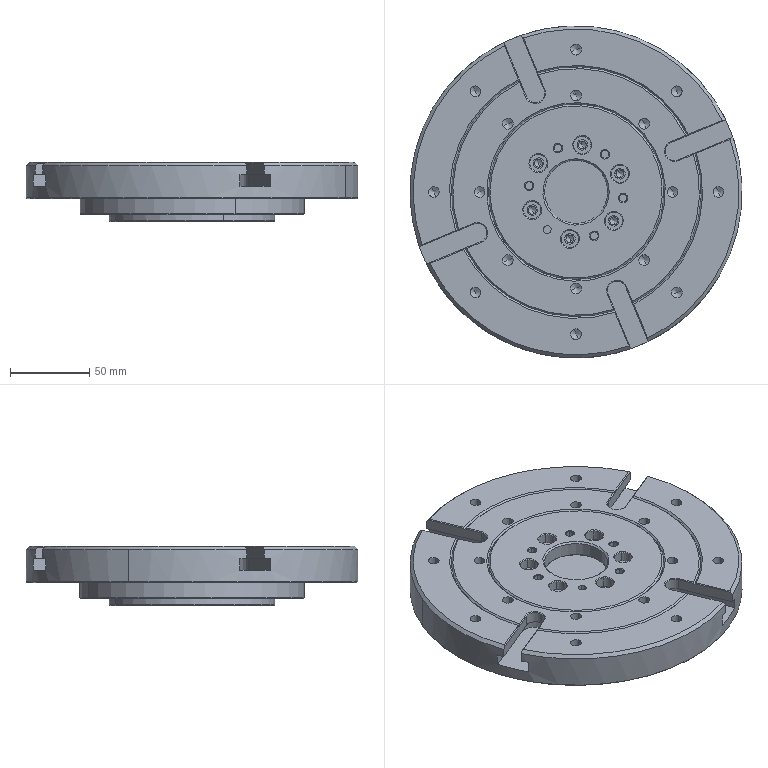NC program | Mastercam | posted with a generic post
Lines 1 to 724 of 4738:
%
:0001()
(MATERIAL - ALUMINUM MM - 2024)
(T1|8 FEMR |H1|XY STOCK TO LEAVE - .1|Z STOCK TO LEAVE - 0.)
(T2|2.5 DR |H2)
(T5|4 FEMR |H5|D5|WEAR COMP|TOOL DIA. - 4.|XY STOCK TO LEAVE - .1|Z STOCK TO LEAVE - .1)
(T6|2 FEMR |H6|D6|WEAR COMP|TOOL DIA. - 2.|XY STOCK TO LEAVE - .1|Z STOCK TO LEAVE - .1)
(T9|8 FEMF |H9|D9|WEAR COMP|TOOL DIA. - 8.)
(T10|12 R0.8 |H10)
(T7|2 FEMF |H7|D7|WEAR COMP|TOOL DIA. - 2.|XY STOCK TO LEAVE - 0.|Z STOCK TO LEAVE - .05)
(T8|6 XXXX |H8|D8|WEAR COMP|TOOL DIA. - 6.)
(T12|5 CHM |H12)
(T13|2.1 DR |H13)
(T11|3 FEM |H11)
(T14|1.95 THML |H14|D14|WEAR COMP|TOOL DIA. - 1.95)
(T15|2.5 BM |H15)
N100 G21
N102 G0 G17 G40 G80 G90 G94 G98
N104 G0 G28 G91 Z0.
N106 G0 G28 X0. Y0.
(8 FEMR |TOOL - 1|DIA. OFF. - 1|LEN. - 1|TOOL DIA. - 8.)
N108 T1 M6
N110 G0 G54 G90 X15.985 Y3.58 C0. B0. S3500 M3
N112 G43 H1 Z50.
N114 Z13.45
N116 G1 Z4.7 F2000.
N118 X15.936 Y3.498
N120 X15.057 Y2.03 Z4.53
N122 G3 X14.809 Y1.274 Z4.45 I1.544 J-.925
N124 X14.755 Y.115 I12.301 J-1.159
N126 X14.754 Y.062 I12.355
N128 G1 Y.045
N130 G2 X14.688 Y-.692 I-4.1
N132 G3 X14.685 Y-.704 I.786 J-.144
N134 G2 X14.583 Y-1.29 I-79.757 J13.658
N136 G1 X14.534 Y-1.568
N138 G2 X14.201 Y-3.41 I-70.503 J11.78
N140 X11.76 Y-8.452 I-16.311 J4.785
N142 X.007 Y-14.474 I-11.753 J8.459
N144 X-14.474 Y.007 J14.481
N146 G1 X-14.473 Y.164
N148 G2 X-13.125 Y6.103 I14.466 J-.163
N150 G3 X-13.06 Y6.318 I-.726 J.338
N152 G2 X-12.476 Y7.877 I4.051 J-.63
N154 G3 X-12.185 Y8.362 I-10.447 J6.598
N156 X-11.954 Y9.123 Z4.53 I-1.564 J.89
N158 G1 X-11.832 Y10.83 Z4.7
N160 X-11.825 Y10.926
N162 G3 X-11.824 Y10.967 I-.578 J.041 F9500.
N164 X-12.403 Y11.546 I-.579
N166 G1 X-12.572 Y11.521
N168 X-12.726 Y11.448
N170 X-12.853 Y11.333
N172 X-12.94 Y11.185
N174 X-14.656 Y6.988
N176 G3 X-15.882 Y.742 I15.291 J-6.246
N178 X.635 Y-15.775 I16.517
N180 X13.322 Y-9.835 J16.517
N182 G1 X18.397 Y-3.748
N184 G3 X18.604 Y-3.177 I-.685 J.571
N186 X18.049 Y-2.351 I-.892
N188 G1 X16.228 Y-1.606
N190 G3 X15.89 Y-1.54 I-.338 J-.826
N192 X15.794 Y-1.545 J-.892
N194 X15.196 Y-1.872 Z4.63 I.096 J-.887 F2000.
N196 G1 X14.561 Y-2.659 Z4.53
N198 G3 X14.21 Y-3.373 Z4.45 I1.401 J-1.13
N200 G2 X13.635 Y-4.705 I-4.119 J.99
N202 G3 X12.835 Y-6.145 I65.029 J-37.097
N204 G2 X9.902 Y-10.045 I-14.708 J8.008
N206 X.013 Y-14.092 I-9.889 J10.06
N208 X-14.024 Y-1.375 J14.107
N210 X-14.09 Y-.001 I14.261 J1.374
N212 X-13.202 Y4.965 I14.327
N214 G3 X-13.102 Y5.426 I-1.008 J.461
N216 G1 Y5.453
N218 G2 X-13.109 Y5.688 I4.093 J.235
N220 X-13.063 Y6.298 I4.1
N222 G3 X-13.043 Y6.566 Z4.477 I-1.78 J.268
N224 X-13.122 Y7.092 Z4.53 I-1.8
N226 G1 X-13.333 Y7.782 Z4.602
N228 G3 X-13.823 Y8.631 Z4.7 I-2.082 J-.637
N230 X-15.415 Y9.323 I-1.592 J-1.486 F9500.
N232 X-17.593 Y7.145 J-2.178
N234 X-17.524 Y6.599 I2.178
N236 G1 X-14.384 Y-5.511
N238 G3 X.129 Y-16.742 I14.513 J3.762
N240 X10.554 Y-12.523 J14.993
N242 G1 X17.819 Y-5.494
N244 G3 X18.35 Y-4.241 I-1.213 J1.253
N246 X16.606 Y-2.497 I-1.744
N248 X15.746 Y-2.725 J-1.744
N250 X15.566 Y-2.842 Z4.679 I.86 J-1.516 F2000.
N252 G1 X14.944 Y-3.304 Z4.602
N254 X14.366 Y-3.735 Z4.53
N256 G3 X13.848 Y-4.339 Z4.45 I1.074 J-1.444
N258 G2 X12.573 Y-6.241 I-14.043 J8.037
N260 X10.665 Y-8.729 I-25.369 J17.475
N262 X4.74 Y-12.861 I-11.024 J9.493
N264 X.004 Y-13.705 I-4.736 J12.867
N266 X-13.707 Y.006 J13.711
N268 X-13.3 Y3.323 I13.711
N270 G3 X-13.018 Y4.55 I-18.218 J4.835
N272 X-13.006 Y4.689 I-.788 J.139
N274 X-13.023 Y4.852 I-.8
N276 G2 X-13.099 Y5.411 I4.014 J.836
N278 G3 X-13.327 Y6.174 Z4.53 I-1.796 J-.121
N280 G1 X-13.682 Y6.802 Z4.602
N282 G3 X-14.375 Y7.491 Z4.7 I-1.568 J-.884
N284 X-15.25 Y7.718 I-.875 J-1.573 F9500.
N286 X-17.05 Y5.918 J-1.8
N288 X-15.916 Y4.246 I1.8
N290 G2 X-14.98 Y3.866 I-2.828 J-8.309
N292 X-14.196 Y2.584 I-.656 J-1.282
N294 X-14.216 Y2.343 I-1.44
N296 G3 X-14.408 Y-.001 I14.212 J-2.344
N298 X-12.532 Y-7.108 I14.404
N300 X-5.285 Y-13.403 I12.529 J7.105
N302 X.004 Y-14.408 I5.289 J13.413
N304 X4.303 Y-13.752 J14.418
N306 X10.983 Y-9.429 I-4.543 J14.343
N308 X12.218 Y-7.943 I-16.026 J14.579
N310 G2 X13.259 Y-7.498 I1.041 J-.996
N312 X13.792 Y-7.601 J-1.441
N314 G1 X14.652 Y-7.944
N316 G3 X15.319 Y-8.072 I.667 J1.672
N318 X17.119 Y-6.272 J1.8
N320 X15.319 Y-4.472 I-1.8
N322 X15.118 Y-4.484 J-1.8
N324 X14.458 Y-4.692 Z4.631 I.201 J-1.788 F2000.
N326 G1 X14.457
N328 X13.567 Y-5.177 Z4.53
N330 G3 X12.97 Y-5.704 Z4.45 I.862 J-1.581
N332 G2 X11.243 Y-7.721 I-13.613 J9.904
N334 X8.946 Y-9.965 I-19.451 J17.622
N336 X2. Y-13.164 I-9.123 J10.667
N338 X.009 Y-13.314 I-1.991 J13.177
N340 X-13.318 Y.013 J13.327
N342 X-13.141 Y2.174 I13.327
N344 G3 X-12.862 Y3.941 I-53.956 J9.427
N346 X-12.852 Y4.089 I-1.056 J.148
N348 X-12.879 Y4.331 I-1.066
N350 X-12.892 Y4.374 I-.771 J-.214
N352 G2 X-13.036 Y4.919 I3.883 J1.314
N354 G3 X-13.355 Y5.649 Z4.53 I-1.768 J-.337
N356 G1 X-13.782 Y6.23 Z4.602
N358 G3 X-14.523 Y6.873 Z4.7 I-1.799 J-1.325
N360 X-15.581 Y7.139 I-1.058 J-1.968 F9500.
N362 X-17.815 Y4.905 J-2.234
N364 X-17.633 Y4.021 I2.234
N366 G1 X-12.823 Y-7.145
N368 G3 X-.363 Y-15.345 I12.46 J5.367
N370 X5.182 Y-14.16 J13.567
N372 G1 X14.845 Y-9.833
N374 G3 X15.952 Y-8.124 I-.766 J1.709
N376 X14.079 Y-6.251 I-1.873
N378 X13.992 Y-6.254 J-1.873
N380 X13.397 Y-6.381 Z4.639 I.087 J-1.87 F2000.
N382 G1 X13.323 Y-6.41 Z4.631
N384 X12.373 Y-6.782 Z4.53
N386 G3 X11.715 Y-7.229 Z4.45 I.656 J-1.676
N388 G2 X9.286 Y-9.362 I-12.429 J11.705
N390 X6.181 Y-11.402 I-12.429 J15.526
N392 X.042 Y-12.918 I-6.139 J11.676
N394 X-3.303 Y-12.487 J13.192
N396 X-12.925 Y.025 I3.324 J12.512
N398 X-12.872 Y1.181 I12.946
N400 X-12.676 Y3.153 I57.239 J-4.709
N402 G3 X-12.659 Y3.573 I-5.098 J.42
N404 G1 Y3.639
N406 G3 X-12.732 Y3.972 I-.8 J-.002
N408 G2 X-12.933 Y4.5 I3.723 J1.716
N410 G3 X-13.326 Y5.192 Z4.53 I-1.722 J-.522
N412 G1 X-13.813 Y5.724 Z4.602
N414 G3 X-14.621 Y6.279 Z4.7 I-1.595 J-1.456
N416 X-15.408 Y6.428 I-.787 J-2.011 F9500.
N418 X-17.568 Y4.268 J-2.16
N420 X-17.361 Y3.346 I2.16
N422 G1 X-12.609 Y-6.723
N424 G3 X.051 Y-14.747 I12.66 J5.976
N426 X3.75 Y-14.249 J14.
N428 G1 X12.922 Y-11.736
N430 G3 X14.291 Y-9.941 I-.492 J1.795
N432 X12.448 Y-8.079 I-1.861
N434 G1 X12.43 Z4.698 F2000.
N436 G3 X12.007 Y-8.127 Z4.656 J-1.862
N438 G1 X11.768 Y-8.183 Z4.631
N440 X10.774 Y-8.415 Z4.53
N442 G3 X10.058 Y-8.763 Z4.45 I.409 J-1.753
N444 G2 X6.628 Y-10.864 I-10.356 J13.056
N446 X2.643 Y-12.266 I-7.316 J14.425
N448 X.076 Y-12.529 I-2.567 J12.388
N450 X-9.18 Y-8.504 J12.651
N452 X-12.525 Y.051 I9.266 J8.555
N454 G1 Y.159
N456 G2 X-12.433 Y2.545 I37.813 J-.258
N458 G3 X-12.427 Y2.811 I-5.555 J.266
N460 X-12.449 Y3.304 I-5.561
N462 X-12.553 Y3.628 I-.796 J-.079
N464 G2 X-12.803 Y4.134 I3.544 J2.06
N466 G3 X-13.26 Y4.785 Z4.53 I-1.665 J-.683
N468 G1 X-13.795 Y5.27 Z4.602
N470 G3 X-14.423 Y5.512 Z4.67 I-.628 J-.695
N472 X-14.718 Y5.465 Z4.7 J-.937
N474 X-15.361 Y4.575 I.295 J-.89 F9500.
N476 X-15.331 Y4.343 I.938
N478 G1 X-13.072 Y-4.467
N480 G3 X-.225 Y-14.436 I12.847 J3.294
N482 X.671 Y-14.405 J13.263
N484 G1 X10.145 Y-13.763
N486 G3 X11.837 Y-11.953 I-.122 J1.81
N488 X10.023 Y-10.139 I-1.814
N490 G1 X10.022
N492 G3 X9.955 Y-10.141 Z4.693 I.001 J-1.814 F2000.
N494 G1 X9.332 Y-10.164 Z4.631
N496 X8.313 Y-10.202 Z4.53
N498 G3 X7.544 Y-10.407 Z4.45 I.067 J-1.799
N500 G2 X.255 Y-12.203 I-7.289 J13.891
N502 X-.041 Y-12.2 J15.687
N504 G3 X-.052 I-.015 J-.8
N506 G2 X-12.204 Y.007 I.055 J12.207
N508 X-12.198 Y.406 I12.207
N510 G3 X-12.175 Y1.862 I-45.35 J1.456
N512 X-12.178 Y2.476 I-45.373
N514 X-12.232 Y3.008 I-3.887 J-.125
N516 X-12.366 Y3.335 I-.789 J-.132
N518 G2 X-12.52 Y3.572 I3.357 J2.353
N520 G3 X-14.062 Y4.443 Z4.634 I-1.542 J-.929
N522 X-14.709 Y4.322 Z4.7 J-1.8
N524 X-15.861 Y2.643 I.647 J-1.679 F9500.
N526 G1 Y2.603
N528 X-15.795 Y-.405
N530 G3 X-13.995 Y-2.165 I1.8 J.04
N532 X-13.636 Y-2.129 J1.8
N534 X-12.195 Y-.365 Z4.455 I-.359 J1.764 F2000.
N536 X-12.196 Y-.318 Z4.45 I-1.8
N538 G2 X-12.2 Y-.016 I12.979 J.302
N540 X-12.05 Y1.946 I12.983
N542 G3 X-12.032 Y2.299 I-3.368 J.353
N544 X-12.067 Y2.787 I-3.386
N546 X-12.228 Y3.149 I-.789 J-.133
N548 G2 X-12.395 Y3.377 I3.219 J2.539
N550 G3 X-13.882 Y4.162 Z4.624 I-1.487 J-1.015
N552 X-14.623 Y4.002 Z4.7 J-1.8
N554 X-15.68 Y2.429 I.741 J-1.64 F9500.
N556 G1 X-15.71 Y1.643
N558 G3 X-15.711 Y1.576 I1.799 J-.067
N560 X-13.911 Y-.224 I1.8
N562 X-13.8 Y-.221 J1.8
N564 X-12.122 Y1.373 Z4.45 I-.111 J1.797 F2000.
N566 G2 X-11.965 Y2.436 I12.067 J-1.248
N568 G3 X-11.963 Y2.509 I-1.387 J.073
N570 X-11.964 Y2.555 I-1.389
N572 X-12.15 Y3.054 I-.799 J-.015
N574 G2 X-12.324 Y3.277 I3.141 J2.634
N576 G3 X-13.775 Y4.018 Z4.618 I-1.456 J-1.059
N578 G1 X-13.818 Z4.623
N580 X-13.823
N582 G3 X-14.574 Y3.854 Z4.7 J-1.8
N584 X-15.623 Y2.218 I.751 J-1.636 F9500.
N586 X-13.823 Y.418 I1.8
N588 G1 X-13.795
N590 G3 X-12.046 Y1.933 Z4.45 I-.028 J1.8 F2000.
N592 G2 X-11.967 Y2.371 I12.046 J-1.933
N594 G3 X-11.952 Y2.527 I-.785 J.156
N596 X-12.141 Y3.043 I-.8
N598 G2 X-12.316 Y3.265 I3.132 J2.645
N600 G3 X-12.917 Y3.787 Z4.582 I-1.451 J-1.064
N602 G1 X-13.552 Y4.128 Z4.7
N604 G0 Z50.
N606 C8.2 B-90.
N608 X11.041 Y14.985
N610 Z3.7
N612 G1 Z1.95
N614 X10.513 Y13.88 Z1.799
N616 G3 X10.337 Y13.104 Z1.7 I1.624 J-.776
N618 G1 Y12.68
N620 X10.512 Y12.622
N622 G3 X12.444 Y12.45 I2.065 J12.237
N624 X14.59 Y12.415 I2.146 J65.36
N626 X15.164 Y12.417 J65.395
N628 X16.558 Y12.999 I-2.379 J7.659
N630 X19.061 Y14.333 I-26.351 J52.475
N632 G2 X20.669 Y14.709 I1.608 J-3.252
N634 X21.522 Y14.607 J-3.628
N636 X24.052 Y12.989 I-1.142 J-4.573
N638 X25.338 Y10.381 I-5.33 J-4.249
N640 X25.75 Y7.488 I-14.543 J-3.548
N642 X25.841 Y3.164 I-102.749 J-4.324
N644 X25.839 Y2.498 I-102.84
N646 X25.841 Y1.364 I-954.811 J-2.057
N648 G1 Y1.081
N650 X25.838 Y-9.636
N652 G2 X24.645 Y-12.31 I-3.883 J.129
N654 X22.082 Y-13.647 I-3.574 J3.729
N656 X20.578 Y-13.793 I-1.504 J7.668
N658 X19.421 Y-13.707 J7.814
N660 X16.494 Y-13.015 I2.801 J18.402
N662 G3 X15.01 Y-12.834 I-1.73 J-8.014
N664 X10.925 Y-12.759 I-4.085 J-110.838
N666 X10.303 Y-12.761 J-110.913
N668 G1 Y-13.043
N670 Y-13.326
N672 G3 X10.479 Y-14.102 Z1.78 I1.8
N674 G1 X11.007 Y-15.206 Z1.902
N676 Y-15.207
N678 G3 X11.273 Y-15.612 Z1.95 I1.624 J.777
N680 X12.631 Y-16.23 I1.358 J1.182
N682 X14.396 Y-14.781 J1.8
N684 G2 X15.827 Y-13.617 I1.431 J-.297 F9500.
N686 X16.267 Y-13.685 J-1.461
N688 X16.843 Y-13.853 I-1.124 J-4.908
N690 G3 X20.003 Y-14.473 I4.458 J14.35
N692 X20.635 Y-14.5 I.632 J7.402
N694 X23.333 Y-13.993 J7.429
N696 X25.956 Y-11.731 I-1.882 J4.834
N698 X26.547 Y-9.436 I-4.159 J2.295
N700 X26.546 Y-9.34 I-4.75
N702 G1 Y-9.088
N704 X26.527 Y5.078
N706 Y5.096
N708 G3 X26.336 Y8.867 I-37.225
N710 X25.554 Y11.878 I-10.177 J-1.035
N712 X23.268 Y14.616 I-5.667 J-2.408
N714 X20.697 Y15.379 I-2.571 J-3.953
N716 X18.321 Y14.737 J-4.716
N718 G2 X16.441 Y13.728 I-30.268 J54.165
N720 X15.795 Y13.575 I-.646 J1.287
N722 X14.404 Y14.642 J1.44
N724 G3 X12.665 Y15.976 I-1.739 J-.466
N726 X11.307 Y15.358 J-1.8
N728 X11.041 Y14.953 Z1.902 I1.358 J-1.182 F2000.
N730 G1 Y14.952
N732 X10.513 Y13.848 Z1.78
N734 G3 X10.337 Y13.072 Z1.7 I1.624 J-.776
N736 G1 Y12.648
N738 Y12.619
N740 G3 X11.174 Y12.384 I1.278 J2.943
N742 X14.104 Y12.173 I2.93 J20.209
N744 X14.539 Y12.178 J20.42
N746 X15.991 Y12.544 I-.447 J4.835
N748 X17.743 Y13.347 I-7.083 J17.753
N750 G2 X19.746 Y13.814 I2.003 J-4.063
N752 X21.757 Y13.343 J-4.53
N754 X24.158 Y11.077 I-2.569 J-5.126
N756 X25.125 Y8.508 I-7.375 J-4.243
N758 X25.493 Y5.135 I-20.138 J-3.904
N760 X25.565 Y-.32 I-207.624 J-5.455
N762 X25.561 Y-1.495 I-207.696
N764 G1 Y-1.778
N766 X25.55 Y-8.343
N768 G2 X23.396 Y-12.003 I-4.835 J.382
N770 X20.237 Y-13.043 I-3.515 J5.359
N772 X19.609 Y-13.062 I-.628 J10.222
N774 X17.847 Y-12.909 J10.241
N776 G1 X17.557 Y-12.867
N778 G3 X12.923 Y-12.514 I-4.762 J-31.888
N780 X11.836 Y-12.497 I-1.087 J-35.399
N782 X10.982 Y-12.507 J-35.416
N784 X10.605 Y-12.551 I.411 J-5.207
N786 G1 X10.303 Y-12.585
N788 Y-13.15
N790 G3 X10.479 Y-13.926 Z1.78 I1.8
N792 G1 X11.007 Y-15.031 Z1.902
N794 G3 X11.253 Y-15.45 Z1.95 I2.597 J1.241
N796 X13.604 Y-16.668 I2.351 J1.66 F9500.
N798 X14.692 Y-16.454 J2.878
N800 G1 X24.149 Y-12.59
N802 G3 X26.706 Y-8.807 I-1.555 J3.806
N804 G1 X26.796 Y7.252
N806 Y7.295
N808 G3 X19.58 Y15.088 I-7.816
N810 G1 X12.253 Y15.652
N812 G3 X12.161 Y15.656 I-.092 J-1.191
N814 X11.304 Y15.294 J-1.195
N816 X11.083 Y14.976 Z1.911 I.857 J-.833 F2000.
N818 G1 X11.041 Y14.889 Z1.902
N820 X10.513 Y13.784 Z1.78
N822 G3 X10.337 Y13.008 Z1.7 I1.624 J-.776
N824 G1 Y12.584
N826 Y12.548
N828 G3 X11.12 Y12.257 I1.381 J2.517
N830 X13.806 Y11.959 I2.686 J11.968
N832 X14.236 Y11.967 J12.266
N834 X16.467 Y12.524 I-.622 J7.233
N836 G2 X17.846 Y13.003 I3.465 J-7.746
N838 X18.975 Y13.127 I1.129 J-5.073
N840 X22.383 Y11.855 J-5.197
N842 X24.324 Y9.072 I-4.511 J-5.216
N844 X25.041 Y6.051 I-11.076 J-4.222
N846 X25.255 Y2.036 I-40.071 J-4.149
N848 X25.281 Y-3.38 I-555.306 J-5.416
N850 X25.268 Y-7.105 I-555.332
N852 X22.358 Y-11.635 I-5.397 J.267
N854 X19.666 Y-12.417 I-3.314 J6.387
N856 X18.261 Y-12.471 I-1.405 J18.136
N858 X16.892 Y-12.42 J18.19
N860 X16.04 Y-12.371 I21.126 J375.776
N862 G3 X11.818 Y-12.241 I-4.236 J-68.925
N864 G1 X11.784
N866 G3 X10.303 Y-12.424 J-6.078
N868 G1 Y-12.706
N870 Y-12.988
N872 G3 X10.479 Y-13.765 Z1.78 I1.8
N874 G1 X11.007 Y-14.869 Z1.902
N876 G3 X11.253 Y-15.288 Z1.95 I2.536 J1.212
N878 X13.543 Y-16.468 I2.29 J1.631 F9500.
N880 X14.648 Y-16.242 J2.811
N882 G1 X23.817 Y-12.325
N884 G3 X26.252 Y-8.805 I-1.578 J3.694
N886 G1 X26.819 Y4.315
N888 G3 X26.829 Y4.783 I-10.828 J.468
N890 X15.991 Y15.622 I-10.838
N892 G1 X11.698
N894 G3 X11.312 Y15.379 J-.427
N896 G1 X11.251 Y15.251
N898 X11.041 Y14.813 Z1.902 F2000.
N900 X10.513 Y13.708 Z1.78
N902 G3 X10.337 Y12.932 Z1.7 I1.624 J-.776
N904 G1 Y12.508
N906 Y12.466
N908 G3 X11.082 Y12.131 I1.472 J2.277
N910 X13.581 Y11.76 I2.499 J8.234
N912 X14.584 Y11.819 J8.605
N914 X16.207 Y12.212 I-1.289 J8.867
N916 G2 X18.274 Y12.562 I2.067 J-5.926
N918 X18.859 Y12.535 J-6.276
N920 X22.695 Y10.457 I-.68 J-5.834
N922 X24.18 Y7.746 I-6.169 J-5.141
N924 X24.805 Y4.526 I-13.995 J-4.388
N926 X24.983 Y.048 I-56.117 J-4.478
N928 G1 Y.009
N930 G2 X24.998 Y-3.343 I-366.192 J-3.352
N932 X24.989 Y-5.963 I-366.207
N934 X23.939 Y-9.22 I-5.985 J.133
N936 X21.026 Y-11.424 I-5. J3.579
N938 X18.126 Y-12.004 I-3.332 J9.128
N940 X16.354 Y-12.043 I-1.772 J40.15
N942 X14.721 Y-12.01 J40.189
N944 G3 X13.112 Y-11.979 I-1.609 J-41.646
N946 X11.888 Y-11.997 J-41.677
N948 X10.303 Y-12.268 I.172 J-5.767
N950 G1 Y-12.551
N952 Y-12.833
N954 G3 X10.479 Y-13.609 Z1.78 I1.8
N956 G1 X11.007 Y-14.714 Z1.902
N958 G3 X11.252 Y-15.133 Z1.95 I2.6 J1.243
N960 X13.607 Y-16.353 I2.355 J1.662 F9500.
N962 X15.023 Y-15.981 J2.882
N964 G1 X23.872 Y-10.988
N966 G3 X25.917 Y-8.036 I-2.023 J3.586
N968 G1 X27.051 Y-.758
N970 G3 X27.22 Y1.43 I-14.043 J2.188
N972 X13.008 Y15.642 I-14.212
N974 X11.709 Y15.583 J-14.212
N976 X11.319 Y15.311 I.044 J-.479
N978 G1 X11.251 Y15.168
N980 X11.041 Y14.729 Z1.902 F2000.
N982 X10.513 Y13.624 Z1.78
N984 G3 X10.337 Y12.848 Z1.7 I1.624 J-.776
N986 G1 Y12.425
N988 Y12.379
N990 G3 X11.048 Y12.008 I1.5 J2.004
N992 X13.616 Y11.574 I2.568 J7.379
N994 X15.449 Y11.792 J7.813
N996 G2 X17.535 Y12.086 I2.284 J-8.634
N998 G1 X17.555
N1000 G2 X22.294 Y9.87 J-6.175
N1002 X23.918 Y6.839 I-6.406 J-5.382
N1004 X24.541 Y3.352 I-15.953 J-4.649
N1006 X24.708 Y-1.502 I-70.401 J-4.854
N1008 G1 Y-1.704
N1010 G2 X24.716 Y-3.28 I-160.75 J-1.576
N1012 X24.707 Y-4.962 I-160.758
N1014 X23.939 Y-7.999 I-6.775 J.097
N1016 X20.925 Y-10.757 I-5.607 J3.102
N1018 X18.052 Y-11.541 I-3.933 J8.749
N1020 X15.165 Y-11.699 I-2.887 J26.274
N1022 X14.81 Y-11.697 J26.432
N1024 G3 X14.159 Y-11.691 I-.651 J-38.204
N1026 X11.985 Y-11.753 J-38.21
N1028 X10.642 Y-11.995 I.388 J-6.01
N1030 X10.303 Y-12.233 I.274 J-.752
N1032 G1 Y-12.515
N1034 G3 X10.479 Y-13.292 Z1.78 I1.8
N1036 G1 X11.007 Y-14.396 Z1.902
N1038 G3 X11.252 Y-14.816 Z1.95 I2.665 J1.274
N1040 X13.672 Y-16.076 I2.42 J1.694 F9500.
N1042 X15.326 Y-15.57 J2.954
N1044 G1 X23.935 Y-9.752
N1046 G3 X25.791 Y-6.318 I-2.363 J3.497
N1048 G1 X25.924 Y2.585
N1050 G3 X25.925 Y2.775 I-12.775 J.19
N1052 X13.149 Y15.551 I-12.776
N1054 X12.456 Y15.532 J-12.776
N1056 X11.331 Y15.029 I.093 J-1.716
N1058 X11.041 Y14.64 Z1.902 I1.218 J-1.213 F2000.
N1060 G1 X10.513 Y13.536 Z1.78
N1062 G3 X10.337 Y12.76 Z1.7 I1.624 J-.776
N1064 G1 Y12.336
N1066 Y12.288
N1068 G3 X11.014 Y11.887 I1.552 J1.848
N1070 X13.639 Y11.384 I2.625 J6.592
N1072 X14.497 Y11.435 J7.095
N1074 X15.531 Y11.576 I-4.452 J36.546
N1076 G2 X16.771 Y11.673 I1.24 J-7.886
N1078 X18.104 Y11.561 J-7.983
N1080 X22.158 Y9.036 I-1.257 J-6.534
N1082 X23.635 Y6.077 I-7.277 J-5.482
N1084 X24.246 Y2.626 I-16.712 J-4.738
N1086 X24.425 Y-2.329 I-68.451 J-4.955
N1088 G1 Y-2.435
N1090 G2 X24.431 Y-3.023 I-27.127 J-.588
N1092 X24.375 Y-4.765 I-27.133
N1094 X20.857 Y-10.097 I-6.589 J.521
N1096 X17.822 Y-11.106 I-4.475 J8.386
N1098 X14.548 Y-11.377 I-3.607 J23.658
N1100 G1 X14.262 Y-11.386
N1102 G3 X11.816 Y-11.54 I.221 J-22.999
N1104 X10.53 Y-11.905 I.394 J-3.839
N1106 X10.303 Y-12.049 I.309 J-.738
N1108 G1 Y-12.331
N1110 G3 X10.479 Y-13.108 Z1.78 I1.8
N1112 G1 X11.007 Y-14.212 Z1.902
N1114 G3 X11.252 Y-14.632 Z1.95 I2.63 J1.257
N1116 X13.637 Y-15.871 I2.385 J1.677 F9500.
N1118 X15.333 Y-15.326 J2.916
N1120 G1 X23.655 Y-9.375
N1122 G3 X25.39 Y-6.221 I-2.423 J3.388
N1124 G1 X25.818 Y1.398
N1126 G3 X25.839 Y2.145 I-13.308 J.747
N1128 X12.51 Y15.474 I-13.329
N1130 X11.313 Y14.949 J-1.628
N1132 X11.041 Y14.548 Z1.902 I1.197 J-1.103 F2000.
N1134 G1 X10.513 Y13.443 Z1.78
N1136 G3 X10.337 Y12.667 Z1.7 I1.624 J-.776
N1138 G1 Y12.243
N1140 Y12.192
N1142 G3 X10.979 Y11.769 I1.58 J1.696
N1144 X13.609 Y11.204 I2.63 J5.84
N1146 X13.782 Y11.206 J6.405
N1148 X15.304 Y11.296 I-.891 J27.859
N1150 G2 X15.982 Y11.323 I.678 J-8.506
N1152 X18.022 Y11.076 J-8.533
N1154 X21.977 Y8.29 I-1.847 J-6.822
N1156 X23.449 Y5.026 I-8.097 J-5.617
N1158 X24.001 Y1.343 I-19.645 J-4.824
N1160 X24.124 Y-2.387 I-56.594 J-3.73
N1162 X24.111 Y-3.591 I-56.717
N1164 X23.233 Y-6.885 I-7.591 J.259
N1166 X20.101 Y-9.833 I-6.19 J3.438
N1168 X17.001 Y-10.793 I-4.651 J9.538
N1170 X13.87 Y-11.095 I-4.688 J32.26
N1172 G3 X11.61 Y-11.358 I.66 J-15.491
N1174 X10.303 Y-11.852 I1.039 J-4.727
N1176 G1 Y-12.134
N1178 Y-12.417
N1180 G3 X10.479 Y-13.193 Z1.78 I1.8
N1182 G1 X11.007 Y-14.298 Z1.902
N1184 G3 X11.25 Y-14.718 Z1.95 I2.813 J1.345
N1186 X13.82 Y-16.071 I2.57 J1.765 F9500.
N1188 X15.968 Y-15.214 J3.118
N1190 G1 X23.813 Y-7.767
N1192 G3 X25.19 Y-4.849 I-3.067 J3.231
N1194 G1 X25.63 Y1.38
N1196 G3 X25.663 Y2.303 I-13.073 J.923
N1198 X12.557 Y15.408 I-13.106
N1200 X11.311 Y14.854 J-1.681
N1202 X11.041 Y14.452 Z1.902 I1.246 J-1.127 F2000.
N1204 G1 X10.513 Y13.347 Z1.78
N1206 G3 X10.337 Y12.571 Z1.7 I1.624 J-.776
N1208 G1 Y12.147
N1210 Y12.093
N1212 G3 X11.076 Y11.585 I1.697 J1.676
N1214 X13.487 Y11.028 I2.546 J5.524
N1216 X14.314 Y11.014 I.827 J24.471
N1218 X15.053 Y11.025 J24.485
N1220 G2 X15.214 Y11.026 I.161 J-8.92
N1222 X17.871 Y10.622 J-8.921
N1224 X21.888 Y7.428 I-2.387 J-7.126
N1226 X23.241 Y4.059 I-9.056 J-5.593
N1228 X23.747 Y.135 I-23.277 J-4.996
N1230 X23.815 Y-1.897 I-30.127 J-2.032
N1232 X23.791 Y-3.107 I-30.195
N1234 X22.778 Y-6.569 I-7.717 J.379
N1236 X19.503 Y-9.515 I-6.412 J3.835
N1238 X16.153 Y-10.51 I-5.033 J10.812
N1240 X13.217 Y-10.86 I-8.083 J55.342
N1242 G3 X11.182 Y-11.28 I.902 J-9.505
N1244 X10.627 Y-11.509 I1.146 J-3.552
N1246 X10.303 Y-11.831 I.377 J-.706
N1248 G1 Y-12.113
N1250 G3 X10.479 Y-12.889 Z1.78 I1.8
N1252 G1 X11.007 Y-13.994 Z1.902
N1254 G3 X11.25 Y-14.415 Z1.95 I2.829 J1.353
N1256 X13.836 Y-15.777 I2.586 J1.774 F9500.
N1258 X16.089 Y-14.823 J3.136
N1260 G1 X23.631 Y-7.037
N1262 G3 X24.889 Y-4.123 I-3.218 J3.117
N1264 G1 X25.081 Y.105
N1266 G3 X25.095 Y.742 I-14.026 J.637
N1268 X17.418 Y13.257 I-14.04
N1270 G1 X13.323 Y15.339
N1272 G3 X12.6 Y15.512 I-.723 J-1.421
N1274 X11.263 Y14.786 J-1.594
N1276 X11.161 Y14.605 Z1.929 I1.337 J-.868 F2000.
N1278 G1 X11.041 Y14.353 Z1.902
N1280 X10.513 Y13.249 Z1.78
N1282 G3 X10.337 Y12.473 Z1.7 I1.624 J-.776
N1284 G1 Y12.049
N1286 Y11.993
N1288 G3 X11.036 Y11.469 I1.691 J1.529
N1290 X13.211 Y10.866 I2.579 J5.072
N1292 X14.785 Y10.769 I2.484 J27.566
N1294 G2 X17.692 Y10.193 I-.399 J-9.643
N1296 X21.536 Y6.998 I-2.854 J-7.344
N1298 X22.944 Y3.492 I-9.404 J-5.812
N1300 X23.47 Y-.757 I-23.828 J-5.107
N1302 X23.495 Y-1.58 I-13.354 J-.823
N1304 X23.374 Y-3.382 I-13.379
N1306 X19.585 Y-8.864 I-7.424 J1.079
N1308 X16.414 Y-10.044 I-5.405 J9.681
N1310 X13.673 Y-10.505 I-7.404 J35.669
N1312 G3 X11.306 Y-11.028 I1.624 J-12.96
N1314 X10.619 Y-11.368 I.875 J-2.63
N1316 X10.303 Y-11.77 I.438 J-.67
N1318 G1 X11.007 Y-11.956 Z1.772
N1320 G3 X12.76 Y-12.283 Z1.95 I3.104 J11.753
N1322 X14.111 Y-12.358 I1.351 J12.08 F9500.
N1324 X26.266 Y-.203 J12.155
N1326 X20.199 Y10.318 I-12.155
N1328 G1 X12.576 Y14.728
N1330 G3 X12.028 Y14.875 I-.548 J-.947
N1332 X11.34 Y14.632 J-1.094
N1334 X11.041 Y14.253 Z1.902 I.688 J-.851 F2000.
N1336 G1 X10.513 Y13.149 Z1.78
N1338 G3 X10.337 Y12.372 Z1.7 I1.624 J-.777
N1340 G1 Y11.949
N1342 Y11.89
N1344 G3 X11.126 Y11.283 I1.866 J1.609
N1346 X13.167 Y10.686 I2.664 J5.316
N1348 G2 X15.201 Y10.434 I-16.008 J-138.038
N1350 X18.541 Y9.243 I-1.244 J-8.767
N1352 X21.605 Y5.873 I-4.476 J-7.145
N1354 X22.789 Y2.281 I-11.623 J-5.825
N1356 X23.134 Y-1.369 I-19.125 J-3.65
N1358 X23.128 Y-1.86 I-19.47
N1360 X22.052 Y-5.677 I-8.152 J.238
N1362 X18.763 Y-8.718 I-6.82 J4.077
N1364 X15.566 Y-9.823 I-5.802 J11.615
N1366 X13.038 Y-10.326 I-14.781 J67.658
N1368 G3 X11.274 Y-10.837 I1.855 J-9.704
N1370 X10.606 Y-11.224 I1.104 J-2.679
N1372 X10.303 Y-11.665 I.47 J-.647
N1374 G1 X11.007 Y-11.804 Z1.771
N1376 G3 X12.788 Y-12.02 Z1.95 I2.329 J11.751
N1378 X13.336 Y-12.033 I.548 J11.967 F9500.
N1380 X25.316 Y-.053 J11.98
N1382 X17.358 Y11.231 I-11.98
N1384 G2 X17.087 Y11.356 I.552 J1.547
N1386 G1 X11.831 Y14.396
N1388 G3 X11.549 Y14.472 I-.282 J-.487
N1390 X11.404 Y14.453 J-.563
N1392 X11.041 Y14.152 Z1.902 I.145 J-.544 F2000.
N1394 G1 X10.513 Y13.047 Z1.78
N1396 G3 X10.337 Y12.271 Z1.7 I1.624 J-.776
N1398 G1 Y11.847
N1400 Y11.787
N1402 G3 X11.085 Y11.168 I1.839 J1.461
N1404 X12.917 Y10.538 I2.756 J5.038
N1406 X14.546 Y10.253 I10.569 J55.602
N1408 G2 X17.65 Y9.22 I-1.618 J-10.04
N1410 X21.137 Y5.725 I-4.161 J-7.639
N1412 X22.42 Y2.141 I-11.18 J-6.025
N1414 X22.76 Y-1.031 I-14.629 J-3.172
N1416 X22.753 Y-1.497 I-14.969
N1418 X21.228 Y-5.944 I-7.987 J.254
N1420 X18.055 Y-8.518 I-6.772 J5.106
N1422 X14.997 Y-9.573 I-6.424 J13.654
N1424 G3 X12.398 Y-10.214 I14.534 J-64.514
N1426 X10.83 Y-10.888 I1.409 J-5.441
N1428 X10.399 Y-11.287 I.671 J-1.158
N1430 X10.303 Y-11.523 I.683 J-.416
N1432 G1 X11.007 Y-11.644 Z1.771
N1434 G3 X12.796 Y-11.81 Z1.95 I1.976 J11.533
N1436 X12.983 Y-11.811 I.187 J11.699 F9500.
N1438 X24.683 Y-.111 J11.7
N1440 X15.664 Y11.278 I-11.7
N1442 G2 X15.19 Y11.514 I.264 J1.123
N1444 G1 X11.913 Y14.24
N1446 G3 X11.551 Y14.371 I-.362 J-.435
N1448 X11.403 Y14.351 J-.566
N1450 X11.041 Y14.049 Z1.902 I.148 J-.546 F2000.
N1452 G1 X10.513 Y12.944 Z1.78
N1454 G3 X10.337 Y12.168 Z1.7 I1.624 J-.776
N1456 G1 Y11.745
N1458 Y11.682
N1460 G3 X11.048 Y11.052 I1.806 J1.322
N1462 X12.677 Y10.404 I2.924 J4.98
N1464 X14.573 Y9.96 I14.853 J59.122
N1466 G2 X17.774 Y8.63 I-2.272 J-9.988
N1468 X20.965 Y5.054 I-4.955 J-7.633
N1470 X22.358 Y-.848 I-11.81 J-5.902
N1472 X22.356 Y-1.077 I-13.203
N1474 X18.821 Y-7.492 I-7.904 J.174
N1476 X15.856 Y-8.925 I-6.571 J9.815
N1478 X13.266 Y-9.685 I-15.858 J49.266
N1480 G3 X11.301 Y-10.411 I2.572 J-9.974
N1482 X10.563 Y-10.923 I1.491 J-2.938
N1484 X10.303 Y-11.367 I.524 J-.605
N1486 G1 X11.007 Y-11.475 Z1.771
N1488 G3 X12.801 Y-11.611 Z1.95 I1.8 J11.839
N1490 G1 X12.807 F9500.
N1492 G3 X24.782 Y.364 J11.975
N1494 X20.074 Y9.882 I-11.975
N1496 G1 X13.411 Y14.969
N1498 G3 X12.556 Y15.257 I-.855 J-1.123
N1500 X11.251 Y14.384 J-1.411
N1502 G1 X11.041 Y13.945 Z1.902 F2000.
N1504 X10.513 Y12.841 Z1.78
N1506 G3 X10.337 Y12.064 Z1.7 I1.624 J-.777
N1508 G1 Y11.641
N1510 Y11.576
N1512 G3 X11.016 Y10.935 I1.955 J1.39